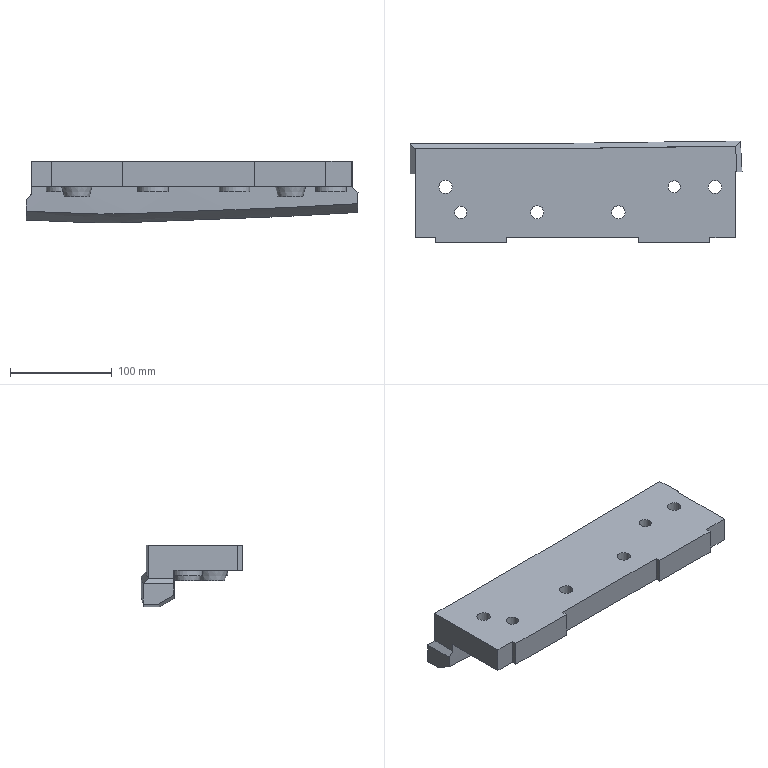Part | NX | features solid 2 | 1 solid | 46 faces | box 326.57 x 100.135 x 60.842 mm | volume 989839 mm3 | plane 26 | cylinder 12 | spline 6 | cone 2 | commonest cylinder face diameters 13 x6 30 x4 12 x2